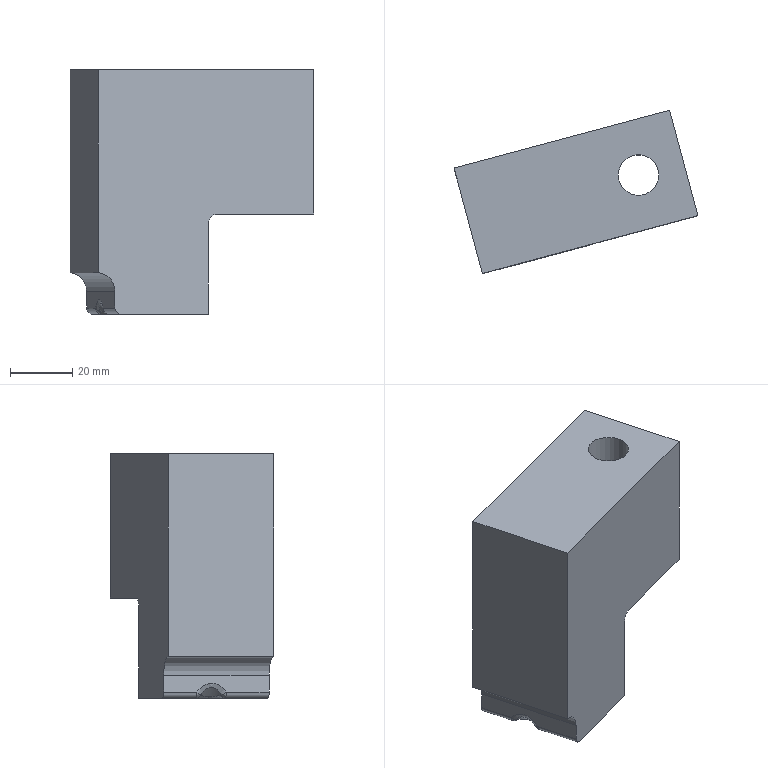Part | NX | features solid 2 | 1 solid | 27 faces | box 78.122 x 52.313 x 78.4 mm | volume 139499 mm3 | plane 12 | cylinder 10 | spline 4 | cone 1 | commonest cylinder face diameters 4 x2 6 x2 8.5 x1 10 x1 11 x1 12 x1
STEP:
#1=CARTESIAN_POINT('',(1284.025,27.373,18.75));
#2=VERTEX_POINT('',#1);
#3=CARTESIAN_POINT('',(1284.025,27.373,65.));
#4=VERTEX_POINT('',#3);
#5=CARTESIAN_POINT('',(1284.025,27.373,142.6));
#6=DIRECTION('',(0.,0.,-1.));
#7=VECTOR('',#6,1000.);
#8=LINE('',#5,#7);
#9=EDGE_CURVE('',#2,#4,#8,.F.);
#10=ORIENTED_EDGE('',*,*,#9,.T.);
#11=CARTESIAN_POINT('',(1214.961,8.867,65.));
#12=VERTEX_POINT('',#11);
#13=CARTESIAN_POINT('',(1303.344,32.549,65.));
#14=DIRECTION('',(-0.9659,-0.2588,0.));
#15=VECTOR('',#14,1000.);
#16=LINE('',#13,#15);
#17=EDGE_CURVE('',#4,#12,#16,.T.);
#18=ORIENTED_EDGE('',*,*,#17,.T.);
#19=CARTESIAN_POINT('',(1214.961,8.867,-0.02087));
#20=VERTEX_POINT('',#19);
#21=CARTESIAN_POINT('',(1214.961,8.867,86.));
#22=DIRECTION('',(0.,0.,1.));
#23=VECTOR('',#22,1000.);
#24=LINE('',#21,#23);
#25=EDGE_CURVE('',#20,#12,#24,.T.);
#26=ORIENTED_EDGE('',*,*,#25,.F.);
#27=CARTESIAN_POINT('',(1220.274,10.291,-6.));
#28=VERTEX_POINT('',#27);
#29=CARTESIAN_POINT('',(1214.478,8.738,-6.));
#30=DIRECTION('',(-0.2588,0.9659,0.));
#31=DIRECTION('',(-0.9659,-0.2588,0.));
#32=AXIS2_PLACEMENT_3D('',#29,#30,#31);
#33=CIRCLE('',#32,6.);
#34=EDGE_CURVE('',#20,#28,#33,.T.);
#35=ORIENTED_EDGE('',*,*,#34,.T.);
#36=CARTESIAN_POINT('',(1220.274,10.291,-11.4));
#37=VERTEX_POINT('',#36);
#38=CARTESIAN_POINT('',(1220.274,10.291,0.));
#39=DIRECTION('',(0.,0.,1.));
#40=VECTOR('',#39,1000.);
#41=LINE('',#38,#40);
#42=EDGE_CURVE('',#28,#37,#41,.F.);
#43=ORIENTED_EDGE('',*,*,#42,.T.);
#44=CARTESIAN_POINT('',(1222.206,10.808,-13.4));
#45=VERTEX_POINT('',#44);
#46=CARTESIAN_POINT('',(1222.206,10.808,-11.4));
#47=DIRECTION('',(-0.2588,0.9659,0.));
#48=DIRECTION('',(-0.9659,-0.2588,0.));
#49=AXIS2_PLACEMENT_3D('',#46,#47,#48);
#50=CIRCLE('',#49,2.);
#51=EDGE_CURVE('',#37,#45,#50,.F.);
#52=ORIENTED_EDGE('',*,*,#51,.T.);
#53=CARTESIAN_POINT('',(1250.218,18.314,-13.4));
#54=VERTEX_POINT('',#53);
#55=CARTESIAN_POINT('',(1303.344,32.549,-13.4));
#56=DIRECTION('',(0.9659,0.2588,0.));
#57=VECTOR('',#56,1000.);
#58=LINE('',#55,#57);
#59=EDGE_CURVE('',#54,#45,#58,.F.);
#60=ORIENTED_EDGE('',*,*,#59,.F.);
#61=CARTESIAN_POINT('',(1250.218,18.314,15.75));
#62=VERTEX_POINT('',#61);
#63=CARTESIAN_POINT('',(1250.218,18.314,142.6));
#64=DIRECTION('',(0.,0.,1.));
#65=VECTOR('',#64,1000.);
#66=LINE('',#63,#65);
#67=EDGE_CURVE('',#54,#62,#66,.T.);
#68=ORIENTED_EDGE('',*,*,#67,.T.);
#69=CARTESIAN_POINT('',(1253.115,19.091,18.75));
#70=VERTEX_POINT('',#69);
#71=CARTESIAN_POINT('',(1253.115,19.091,15.75));
#72=DIRECTION('',(0.2588,-0.9659,0.));
#73=DIRECTION('',(0.9659,0.2588,0.));
#74=AXIS2_PLACEMENT_3D('',#71,#72,#73);
#75=CIRCLE('',#74,3.);
#76=EDGE_CURVE('',#62,#70,#75,.F.);
#77=ORIENTED_EDGE('',*,*,#76,.T.);
#78=CARTESIAN_POINT('',(1303.344,32.549,18.75));
#79=DIRECTION('',(0.9659,0.2588,0.));
#80=VECTOR('',#79,1000.);
#81=LINE('',#78,#80);
#82=EDGE_CURVE('',#2,#70,#81,.F.);
#83=ORIENTED_EDGE('',*,*,#82,.F.);
#84=EDGE_LOOP('',(#10,#18,#26,#35,#43,#52,#60,#68,#77,#83));
#85=FACE_BOUND('',#84,.T.);
#86=CARTESIAN_POINT('',(1303.344,32.549,-6.));
#87=DIRECTION('',(0.2588,-0.9659,0.));
#88=DIRECTION('',(-0.9659,-0.2588,0.));
#89=AXIS2_PLACEMENT_3D('',#86,#87,#88);
#90=PLANE('',#89);
#91=ADVANCED_FACE('',(#85),#90,.T.);
#92=ORIENTED_EDGE('',*,*,#25,.T.);
#93=CARTESIAN_POINT('',(1205.903,42.675,65.));
#94=VERTEX_POINT('',#93);
#95=CARTESIAN_POINT('',(1203.025,53.415,65.));
#96=DIRECTION('',(-0.2588,0.9659,0.));
#97=VECTOR('',#96,1000.);
#98=LINE('',#95,#97);
#99=EDGE_CURVE('',#12,#94,#98,.T.);
#100=ORIENTED_EDGE('',*,*,#99,.T.);
#101=CARTESIAN_POINT('',(1205.903,42.675,-0.02087));
#102=VERTEX_POINT('',#101);
#103=CARTESIAN_POINT('',(1205.903,42.675,181.6));
#104=DIRECTION('',(0.,0.,-1.));
#105=VECTOR('',#104,1000.);
#106=LINE('',#103,#105);
#107=EDGE_CURVE('',#94,#102,#106,.T.);
#108=ORIENTED_EDGE('',*,*,#107,.T.);
#109=CARTESIAN_POINT('',(1215.168,8.097,-0.02087));
#110=DIRECTION('',(0.2588,-0.9659,0.));
#111=VECTOR('',#110,1000.);
#112=LINE('',#109,#111);
#113=EDGE_CURVE('',#20,#102,#112,.F.);
#114=ORIENTED_EDGE('',*,*,#113,.F.);
#115=EDGE_LOOP('',(#92,#100,#108,#114));
#116=FACE_BOUND('',#115,.T.);
#117=CARTESIAN_POINT('',(1203.025,53.415,86.));
#118=DIRECTION('',(-0.9659,-0.2588,0.));
#119=DIRECTION('',(-0.2588,0.9659,0.));
#120=AXIS2_PLACEMENT_3D('',#117,#118,#119);
#121=PLANE('',#120);
#122=ADVANCED_FACE('',(#116),#121,.T.);
#123=CARTESIAN_POINT('',(1274.966,61.18,65.));
#124=VERTEX_POINT('',#123);
#125=CARTESIAN_POINT('',(1213.147,44.616,65.));
#126=DIRECTION('',(-0.9659,-0.2588,0.));
#127=VECTOR('',#126,1000.);
#128=LINE('',#125,#127);
#129=EDGE_CURVE('',#124,#94,#128,.T.);
#130=ORIENTED_EDGE('',*,*,#129,.F.);
#131=CARTESIAN_POINT('',(1274.966,61.18,18.75));
#132=VERTEX_POINT('',#131);
#133=CARTESIAN_POINT('',(1274.966,61.18,142.6));
#134=DIRECTION('',(0.,0.,-1.));
#135=VECTOR('',#134,1000.);
#136=LINE('',#133,#135);
#137=EDGE_CURVE('',#132,#124,#136,.F.);
#138=ORIENTED_EDGE('',*,*,#137,.F.);
#139=CARTESIAN_POINT('',(1244.057,52.898,18.75));
#140=VERTEX_POINT('',#139);
#141=CARTESIAN_POINT('',(1213.147,44.616,18.75));
#142=DIRECTION('',(0.9659,0.2588,0.));
#143=VECTOR('',#142,1000.);
#144=LINE('',#141,#143);
#145=EDGE_CURVE('',#132,#140,#144,.F.);
#146=ORIENTED_EDGE('',*,*,#145,.T.);
#147=CARTESIAN_POINT('',(1241.159,52.122,15.75));
#148=VERTEX_POINT('',#147);
#149=CARTESIAN_POINT('',(1244.057,52.898,15.75));
#150=DIRECTION('',(0.2588,-0.9659,0.));
#151=DIRECTION('',(0.9659,0.2588,0.));
#152=AXIS2_PLACEMENT_3D('',#149,#150,#151);
#153=CIRCLE('',#152,3.);
#154=EDGE_CURVE('',#140,#148,#153,.T.);
#155=ORIENTED_EDGE('',*,*,#154,.T.);
#156=CARTESIAN_POINT('',(1241.159,52.122,-13.4));
#157=VERTEX_POINT('',#156);
#158=CARTESIAN_POINT('',(1241.159,52.122,142.6));
#159=DIRECTION('',(0.,0.,1.));
#160=VECTOR('',#159,1000.);
#161=LINE('',#158,#160);
#162=EDGE_CURVE('',#157,#148,#161,.T.);
#163=ORIENTED_EDGE('',*,*,#162,.F.);
#164=CARTESIAN_POINT('',(1213.147,44.616,-13.4));
#165=VERTEX_POINT('',#164);
#166=CARTESIAN_POINT('',(1211.215,44.098,-13.4));
#167=DIRECTION('',(-0.9659,-0.2588,0.));
#168=VECTOR('',#167,1000.);
#169=LINE('',#166,#168);
#170=EDGE_CURVE('',#157,#165,#169,.T.);
#171=ORIENTED_EDGE('',*,*,#170,.T.);
#172=CARTESIAN_POINT('',(1211.215,44.098,-11.4));
#173=VERTEX_POINT('',#172);
#174=CARTESIAN_POINT('',(1213.147,44.616,-11.4));
#175=DIRECTION('',(-0.2588,0.9659,0.));
#176=DIRECTION('',(-0.9659,-0.2588,0.));
#177=AXIS2_PLACEMENT_3D('',#174,#175,#176);
#178=CIRCLE('',#177,2.);
#179=EDGE_CURVE('',#173,#165,#178,.F.);
#180=ORIENTED_EDGE('',*,*,#179,.F.);
#181=CARTESIAN_POINT('',(1211.215,44.098,-6.));
#182=VERTEX_POINT('',#181);
#183=CARTESIAN_POINT('',(1211.215,44.098,0.));
#184=DIRECTION('',(0.,0.,1.));
#185=VECTOR('',#184,1000.);
#186=LINE('',#183,#185);
#187=EDGE_CURVE('',#173,#182,#186,.T.);
#188=ORIENTED_EDGE('',*,*,#187,.T.);
#189=CARTESIAN_POINT('',(1205.42,42.545,-6.));
#190=DIRECTION('',(-0.2588,0.9659,0.));
#191=DIRECTION('',(-0.9659,-0.2588,0.));
#192=AXIS2_PLACEMENT_3D('',#189,#190,#191);
#193=CIRCLE('',#192,6.);
#194=EDGE_CURVE('',#182,#102,#193,.F.);
#195=ORIENTED_EDGE('',*,*,#194,.T.);
#196=ORIENTED_EDGE('',*,*,#107,.F.);
#197=EDGE_LOOP('',(#130,#138,#146,#155,#163,#171,#180,#188,#195,#196));
#198=FACE_BOUND('',#197,.T.);
#199=CARTESIAN_POINT('',(1213.147,44.616,181.6));
#200=DIRECTION('',(0.2588,-0.9659,0.));
#201=DIRECTION('',(-0.9659,-0.2588,0.));
#202=AXIS2_PLACEMENT_3D('',#199,#200,#201);
#203=PLANE('',#202);
#204=ADVANCED_FACE('',(#198),#203,.F.);
#205=ORIENTED_EDGE('',*,*,#137,.T.);
#206=CARTESIAN_POINT('',(1284.231,26.602,65.));
#207=DIRECTION('',(0.2588,-0.9659,0.));
#208=VECTOR('',#207,1000.);
#209=LINE('',#206,#208);
#210=EDGE_CURVE('',#124,#4,#209,.T.);
#211=ORIENTED_EDGE('',*,*,#210,.T.);
#212=ORIENTED_EDGE('',*,*,#9,.F.);
#213=CARTESIAN_POINT('',(1284.231,26.602,18.75));
#214=DIRECTION('',(-0.2588,0.9659,0.));
#215=VECTOR('',#214,1000.);
#216=LINE('',#213,#215);
#217=EDGE_CURVE('',#132,#2,#216,.F.);
#218=ORIENTED_EDGE('',*,*,#217,.F.);
#219=EDGE_LOOP('',(#205,#211,#212,#218));
#220=FACE_BOUND('',#219,.T.);
#221=CARTESIAN_POINT('',(1284.231,26.602,142.6));
#222=DIRECTION('',(0.9659,0.2588,0.));
#223=DIRECTION('',(0.2588,-0.9659,0.));
#224=AXIS2_PLACEMENT_3D('',#221,#222,#223);
#225=PLANE('',#224);
#226=ADVANCED_FACE('',(#220),#225,.T.);
#227=CARTESIAN_POINT('',(1271.507,40.394,48.));
#228=VERTEX_POINT('',#227);
#229=CARTESIAN_POINT('',(1265.007,40.394,48.));
#230=DIRECTION('',(0.,0.,1.));
#231=DIRECTION('',(1.,0.,0.));
#232=AXIS2_PLACEMENT_3D('',#229,#230,#231);
#233=CIRCLE('',#232,6.5);
#234=EDGE_CURVE('',#228,#228,#233,.F.);
#235=ORIENTED_EDGE('',*,*,#234,.T.);
#236=EDGE_LOOP('',(#235));
#237=FACE_BOUND('',#236,.T.);
#238=CARTESIAN_POINT('',(1271.507,40.394,65.));
#239=VERTEX_POINT('',#238);
#240=CARTESIAN_POINT('',(1265.007,40.394,65.));
#241=DIRECTION('',(0.,0.,1.));
#242=DIRECTION('',(1.,0.,0.));
#243=AXIS2_PLACEMENT_3D('',#240,#241,#242);
#244=CIRCLE('',#243,6.5);
#245=EDGE_CURVE('',#239,#239,#244,.F.);
#246=ORIENTED_EDGE('',*,*,#245,.F.);
#247=EDGE_LOOP('',(#246));
#248=FACE_BOUND('',#247,.T.);
#249=CARTESIAN_POINT('',(1265.007,40.394,53.75));
#250=DIRECTION('',(0.,0.,1.));
#251=DIRECTION('',(1.,0.,0.));
#252=AXIS2_PLACEMENT_3D('',#249,#250,#251);
#253=CYLINDRICAL_SURFACE('',#252,6.5);
#254=ADVANCED_FACE('',(#237,#248),#253,.F.);
#255=CARTESIAN_POINT('',(1247.014,30.269,15.75));
#256=VERTEX_POINT('',#255);
#257=CARTESIAN_POINT('',(1247.014,30.269,-13.4));
#258=VERTEX_POINT('',#257);
#259=CARTESIAN_POINT('',(1247.014,30.269,18.75));
#260=DIRECTION('',(0.,0.,-1.));
#261=VECTOR('',#260,1000.);
#262=LINE('',#259,#261);
#263=EDGE_CURVE('',#256,#258,#262,.T.);
#264=ORIENTED_EDGE('',*,*,#263,.F.);
#265=CARTESIAN_POINT('',(1250.424,17.544,15.75));
#266=DIRECTION('',(-0.2588,0.9659,0.));
#267=VECTOR('',#266,1000.);
#268=LINE('',#265,#267);
#269=EDGE_CURVE('',#256,#62,#268,.F.);
#270=ORIENTED_EDGE('',*,*,#269,.T.);
#271=ORIENTED_EDGE('',*,*,#67,.F.);
#272=CARTESIAN_POINT('',(1242.3,47.861,-13.4));
#273=DIRECTION('',(0.2588,-0.9659,0.));
#274=VECTOR('',#273,1000.);
#275=LINE('',#272,#274);
#276=EDGE_CURVE('',#258,#54,#275,.T.);
#277=ORIENTED_EDGE('',*,*,#276,.F.);
#278=EDGE_LOOP('',(#264,#270,#271,#277));
#279=FACE_BOUND('',#278,.T.);
#280=CARTESIAN_POINT('',(1250.424,17.544,142.6));
#281=DIRECTION('',(0.9659,0.2588,0.));
#282=DIRECTION('',(0.2588,-0.9659,0.));
#283=AXIS2_PLACEMENT_3D('',#280,#281,#282);
#284=PLANE('',#283);
#285=ADVANCED_FACE('',(#279),#284,.T.);
#286=ORIENTED_EDGE('',*,*,#162,.T.);
#287=CARTESIAN_POINT('',(1244.362,40.167,15.75));
#288=VERTEX_POINT('',#287);
#289=CARTESIAN_POINT('',(1250.424,17.544,15.75));
#290=DIRECTION('',(-0.2588,0.9659,0.));
#291=VECTOR('',#290,1000.);
#292=LINE('',#289,#291);
#293=EDGE_CURVE('',#148,#288,#292,.F.);
#294=ORIENTED_EDGE('',*,*,#293,.T.);
#295=CARTESIAN_POINT('',(1244.362,40.167,-13.4));
#296=VERTEX_POINT('',#295);
#297=CARTESIAN_POINT('',(1244.362,40.167,-13.4));
#298=DIRECTION('',(0.,0.,-1.));
#299=VECTOR('',#298,1000.);
#300=LINE('',#297,#299);
#301=EDGE_CURVE('',#296,#288,#300,.F.);
#302=ORIENTED_EDGE('',*,*,#301,.F.);
#303=CARTESIAN_POINT('',(1242.3,47.861,-13.4));
#304=DIRECTION('',(0.2588,-0.9659,0.));
#305=VECTOR('',#304,1000.);
#306=LINE('',#303,#305);
#307=EDGE_CURVE('',#157,#296,#306,.T.);
#308=ORIENTED_EDGE('',*,*,#307,.F.);
#309=EDGE_LOOP('',(#286,#294,#302,#308));
#310=FACE_BOUND('',#309,.T.);
#311=CARTESIAN_POINT('',(1250.424,17.544,142.6));
#312=DIRECTION('',(0.9659,0.2588,0.));
#313=DIRECTION('',(0.2588,-0.9659,0.));
#314=AXIS2_PLACEMENT_3D('',#311,#312,#313);
#315=PLANE('',#314);
#316=ADVANCED_FACE('',(#310),#315,.T.);
#317=CARTESIAN_POINT('',(1217.195,25.606,-12.41));
#318=VERTEX_POINT('',#317);
#319=CARTESIAN_POINT('',(1216.601,23.998,-11.4));
#320=VERTEX_POINT('',#319);
#321=CARTESIAN_POINT('',(1217.195,25.606,-12.41));
#322=CARTESIAN_POINT('',(1217.092,25.518,-12.368));
#323=CARTESIAN_POINT('',(1216.836,25.249,-12.228));
#324=CARTESIAN_POINT('',(1216.559,24.723,-11.913));
#325=CARTESIAN_POINT('',(1216.534,24.249,-11.588));
#326=CARTESIAN_POINT('',(1216.601,23.998,-11.4));
#327=B_SPLINE_CURVE_WITH_KNOTS('',3,(#321,#322,#323,#324,#325,#326),.UNSPECIFIED.,.F.,.F.,(4,1,1,4),(0.,0.25,0.5,1.),.UNSPECIFIED.);
#328=EDGE_CURVE('',#318,#320,#327,.T.);
#329=ORIENTED_EDGE('',*,*,#328,.F.);
#330=CARTESIAN_POINT('',(1218.533,24.515,-13.4));
#331=VERTEX_POINT('',#330);
#332=CARTESIAN_POINT('',(1218.533,24.515,-13.4));
#333=CARTESIAN_POINT('',(1218.423,24.605,-13.4));
#334=CARTESIAN_POINT('',(1218.117,24.854,-13.353));
#335=CARTESIAN_POINT('',(1217.758,25.147,-13.159));
#336=CARTESIAN_POINT('',(1217.421,25.422,-12.819));
#337=CARTESIAN_POINT('',(1217.28,25.537,-12.597));
#338=CARTESIAN_POINT('',(1217.195,25.606,-12.41));
#339=B_SPLINE_CURVE_WITH_KNOTS('',3,(#332,#333,#334,#335,#336,#337,#338),.UNSPECIFIED.,.F.,.F.,(4,1,1,1,4),(0.,0.25,0.5,0.75,1.),.UNSPECIFIED.);
#340=EDGE_CURVE('',#318,#331,#339,.F.);
#341=ORIENTED_EDGE('',*,*,#340,.T.);
#342=CARTESIAN_POINT('',(1218.533,24.515,-11.4));
#343=DIRECTION('',(0.2588,-0.9659,0.));
#344=DIRECTION('',(-0.9659,-0.2588,0.));
#345=AXIS2_PLACEMENT_3D('',#342,#343,#344);
#346=CIRCLE('',#345,2.);
#347=EDGE_CURVE('',#331,#320,#346,.F.);
#348=ORIENTED_EDGE('',*,*,#347,.T.);
#349=EDGE_LOOP('',(#329,#341,#348));
#350=FACE_BOUND('',#349,.T.);
#351=CARTESIAN_POINT('',(1218.548,23.887,-13.299));
#352=CARTESIAN_POINT('',(1218.458,24.219,-13.409));
#353=CARTESIAN_POINT('',(1218.515,24.574,-13.431));
#354=CARTESIAN_POINT('',(1218.706,24.871,-13.36));
#355=CARTESIAN_POINT('',(1217.473,23.62,-13.219));
#356=CARTESIAN_POINT('',(1217.302,24.242,-13.426));
#357=CARTESIAN_POINT('',(1217.41,24.91,-13.468));
#358=CARTESIAN_POINT('',(1217.77,25.469,-13.335));
#359=CARTESIAN_POINT('',(1216.682,23.663,-12.44));
#360=CARTESIAN_POINT('',(1216.488,24.372,-12.676));
#361=CARTESIAN_POINT('',(1216.61,25.134,-12.723));
#362=CARTESIAN_POINT('',(1217.021,25.77,-12.571));
#363=CARTESIAN_POINT('',(1216.602,23.993,-11.382));
#364=CARTESIAN_POINT('',(1216.453,24.538,-11.563));
#365=CARTESIAN_POINT('',(1216.547,25.123,-11.6));
#366=CARTESIAN_POINT('',(1216.863,25.612,-11.483));
#367=(BOUNDED_SURFACE()B_SPLINE_SURFACE(3,3,((#351,#352,#353,#354),(#355,#356,#357,#358),(#359,#360,#361,#362),(#363,#364,#365,#366)),.UNSPECIFIED.,.F.,.F.,.F.)B_SPLINE_SURFACE_WITH_KNOTS((4,4),(4,4),(0.0005941,0.9994),(0.000239,0.9998),.PIECEWISE_BEZIER_KNOTS.)GEOMETRIC_REPRESENTATION_ITEM()RATIONAL_B_SPLINE_SURFACE(((0.9996,0.9224,0.9224,0.9996),(0.8197,0.7563,0.7563,0.8197),(0.8197,0.7563,0.7563,0.8197),(0.9996,0.9224,0.9224,0.9996)))REPRESENTATION_ITEM('')SURFACE());
#368=ADVANCED_FACE('',(#350),#367,.T.);
#369=CARTESIAN_POINT('',(1218.631,29.613,-12.814));
#370=VERTEX_POINT('',#369);
#371=CARTESIAN_POINT('',(1217.195,25.606,-12.41));
#372=CARTESIAN_POINT('',(1217.496,25.918,-12.472));
#373=CARTESIAN_POINT('',(1218.01,26.568,-12.582));
#374=CARTESIAN_POINT('',(1218.487,27.429,-12.697));
#375=CARTESIAN_POINT('',(1218.791,28.607,-12.796));
#376=CARTESIAN_POINT('',(1218.719,29.284,-12.814));
#377=CARTESIAN_POINT('',(1218.631,29.613,-12.814));
#378=B_SPLINE_CURVE_WITH_KNOTS('',3,(#371,#372,#373,#374,#375,#376,#377),.UNSPECIFIED.,.F.,.F.,(4,1,1,1,4),(0.000000039,0.25,0.5,0.75,1.),.UNSPECIFIED.);
#379=EDGE_CURVE('',#370,#318,#378,.F.);
#380=ORIENTED_EDGE('',*,*,#379,.T.);
#381=CARTESIAN_POINT('',(1215.899,28.881,-9.986));
#382=VERTEX_POINT('',#381);
#383=CARTESIAN_POINT('',(1215.899,28.881,-9.986));
#384=CARTESIAN_POINT('',(1215.99,28.54,-9.986));
#385=CARTESIAN_POINT('',(1216.196,27.854,-10.113));
#386=CARTESIAN_POINT('',(1216.544,26.924,-10.685));
#387=CARTESIAN_POINT('',(1216.844,26.251,-11.376));
#388=CARTESIAN_POINT('',(1217.077,25.806,-12.039));
#389=CARTESIAN_POINT('',(1217.195,25.606,-12.41));
#390=B_SPLINE_CURVE_WITH_KNOTS('',3,(#383,#384,#385,#386,#387,#388,#389),.UNSPECIFIED.,.F.,.F.,(4,1,1,1,4),(0.,0.25,0.5,0.75,1.),.UNSPECIFIED.);
#391=EDGE_CURVE('',#382,#318,#390,.T.);
#392=ORIENTED_EDGE('',*,*,#391,.F.);
#393=CARTESIAN_POINT('',(1215.384,32.366,-12.41));
#394=VERTEX_POINT('',#393);
#395=CARTESIAN_POINT('',(1215.899,28.881,-9.986));
#396=CARTESIAN_POINT('',(1215.716,29.563,-9.986));
#397=CARTESIAN_POINT('',(1215.439,30.969,-10.562));
#398=CARTESIAN_POINT('',(1215.38,31.927,-11.708));
#399=CARTESIAN_POINT('',(1215.384,32.366,-12.41));
#400=B_SPLINE_CURVE_WITH_KNOTS('',3,(#395,#396,#397,#398,#399),.UNSPECIFIED.,.F.,.F.,(4,1,4),(0.,0.5,1.),.UNSPECIFIED.);
#401=EDGE_CURVE('',#394,#382,#400,.F.);
#402=ORIENTED_EDGE('',*,*,#401,.F.);
#403=CARTESIAN_POINT('',(1218.631,29.613,-12.814));
#404=CARTESIAN_POINT('',(1218.543,29.942,-12.814));
#405=CARTESIAN_POINT('',(1218.266,30.564,-12.796));
#406=CARTESIAN_POINT('',(1217.414,31.433,-12.697));
#407=CARTESIAN_POINT('',(1216.571,31.94,-12.582));
#408=CARTESIAN_POINT('',(1215.801,32.246,-12.472));
#409=CARTESIAN_POINT('',(1215.384,32.366,-12.41));
#410=B_SPLINE_CURVE_WITH_KNOTS('',3,(#403,#404,#405,#406,#407,#408,#409),.UNSPECIFIED.,.F.,.F.,(4,1,1,1,4),(0.,0.25,0.5,0.75,1.),.UNSPECIFIED.);
#411=EDGE_CURVE('',#394,#370,#410,.F.);
#412=ORIENTED_EDGE('',*,*,#411,.T.);
#413=EDGE_LOOP('',(#380,#392,#402,#412));
#414=FACE_BOUND('',#413,.T.);
#415=CARTESIAN_POINT('',(1213.815,28.323,-14.899));
#416=DIRECTION('',(-0.683,-0.183,0.7071));
#417=DIRECTION('',(-0.683,-0.183,-0.7071));
#418=AXIS2_PLACEMENT_3D('',#415,#416,#417);
#419=CYLINDRICAL_SURFACE('',#418,5.);
#420=ADVANCED_FACE('',(#414),#419,.F.);
#421=CARTESIAN_POINT('',(1214.065,33.462,-11.4));
#422=VERTEX_POINT('',#421);
#423=CARTESIAN_POINT('',(1214.065,33.462,-11.4));
#424=CARTESIAN_POINT('',(1214.095,33.351,-11.483));
#425=CARTESIAN_POINT('',(1214.223,33.054,-11.714));
#426=CARTESIAN_POINT('',(1214.507,32.741,-11.985));
#427=CARTESIAN_POINT('',(1214.927,32.488,-12.24));
#428=CARTESIAN_POINT('',(1215.18,32.403,-12.346));
#429=CARTESIAN_POINT('',(1215.384,32.366,-12.41));
#430=B_SPLINE_CURVE_WITH_KNOTS('',3,(#423,#424,#425,#426,#427,#428,#429),.UNSPECIFIED.,.F.,.F.,(4,1,1,1,4),(0.,0.25,0.5,0.75,1.),.UNSPECIFIED.);
#431=EDGE_CURVE('',#422,#394,#430,.T.);
#432=ORIENTED_EDGE('',*,*,#431,.F.);
#433=CARTESIAN_POINT('',(1215.997,33.979,-13.4));
#434=VERTEX_POINT('',#433);
#435=CARTESIAN_POINT('',(1215.997,33.979,-11.4));
#436=DIRECTION('',(-0.2588,0.9659,0.));
#437=DIRECTION('',(-0.9659,-0.2588,0.));
#438=AXIS2_PLACEMENT_3D('',#435,#436,#437);
#439=CIRCLE('',#438,2.);
#440=EDGE_CURVE('',#422,#434,#439,.F.);
#441=ORIENTED_EDGE('',*,*,#440,.T.);
#442=CARTESIAN_POINT('',(1215.384,32.366,-12.41));
#443=CARTESIAN_POINT('',(1215.409,32.432,-12.532));
#444=CARTESIAN_POINT('',(1215.494,32.656,-12.849));
#445=CARTESIAN_POINT('',(1215.685,33.159,-13.253));
#446=CARTESIAN_POINT('',(1215.883,33.679,-13.4));
#447=CARTESIAN_POINT('',(1215.997,33.979,-13.4));
#448=B_SPLINE_CURVE_WITH_KNOTS('',3,(#442,#443,#444,#445,#446,#447),.UNSPECIFIED.,.F.,.F.,(4,1,1,4),(0.,0.25,0.5,1.),.UNSPECIFIED.);
#449=EDGE_CURVE('',#434,#394,#448,.F.);
#450=ORIENTED_EDGE('',*,*,#449,.T.);
#451=EDGE_LOOP('',(#432,#441,#450));
#452=FACE_BOUND('',#451,.T.);
#453=CARTESIAN_POINT('',(1214.005,34.078,-11.546));
#454=CARTESIAN_POINT('',(1213.987,33.718,-11.548));
#455=CARTESIAN_POINT('',(1214.051,33.395,-11.401));
#456=CARTESIAN_POINT('',(1214.181,33.184,-11.139));
#457=CARTESIAN_POINT('',(1214.086,34.079,-12.656));
#458=CARTESIAN_POINT('',(1214.053,33.402,-12.659));
#459=CARTESIAN_POINT('',(1214.173,32.794,-12.383));
#460=CARTESIAN_POINT('',(1214.417,32.397,-11.89));
#461=CARTESIAN_POINT('',(1214.904,34.043,-13.41));
#462=CARTESIAN_POINT('',(1214.866,33.271,-13.414));
#463=CARTESIAN_POINT('',(1215.002,32.578,-13.098));
#464=CARTESIAN_POINT('',(1215.281,32.126,-12.536));
#465=CARTESIAN_POINT('',(1216.015,33.989,-13.4));
#466=CARTESIAN_POINT('',(1215.986,33.396,-13.403));
#467=CARTESIAN_POINT('',(1216.091,32.864,-13.161));
#468=CARTESIAN_POINT('',(1216.305,32.517,-12.729));
#469=(BOUNDED_SURFACE()B_SPLINE_SURFACE(3,3,((#453,#454,#455,#456),(#457,#458,#459,#460),(#461,#462,#463,#464),(#465,#466,#467,#468)),.UNSPECIFIED.,.F.,.F.,.F.)B_SPLINE_SURFACE_WITH_KNOTS((4,4),(4,4),(0.,1.),(0.,1.),.PIECEWISE_BEZIER_KNOTS.)GEOMETRIC_REPRESENTATION_ITEM()RATIONAL_B_SPLINE_SURFACE(((1.,0.9226,0.9226,1.),(0.8196,0.7562,0.7562,0.8196),(0.8196,0.7562,0.7562,0.8196),(1.,0.9226,0.9226,1.)))REPRESENTATION_ITEM('')SURFACE());
#470=ADVANCED_FACE('',(#452),#469,.T.);
#471=ORIENTED_EDGE('',*,*,#431,.T.);
#472=ORIENTED_EDGE('',*,*,#401,.T.);
#473=ORIENTED_EDGE('',*,*,#391,.T.);
#474=ORIENTED_EDGE('',*,*,#328,.T.);
#475=CARTESIAN_POINT('',(1214.065,33.462,-11.4));
#476=CARTESIAN_POINT('',(1214.141,33.181,-10.997));
#477=CARTESIAN_POINT('',(1214.303,32.574,-10.273));
#478=CARTESIAN_POINT('',(1214.581,31.538,-9.387));
#479=CARTESIAN_POINT('',(1214.975,30.067,-8.69));
#480=CARTESIAN_POINT('',(1215.325,28.758,-8.504));
#481=CARTESIAN_POINT('',(1215.724,27.272,-8.723));
#482=CARTESIAN_POINT('',(1216.189,25.536,-9.585));
#483=CARTESIAN_POINT('',(1216.451,24.557,-10.597));
#484=CARTESIAN_POINT('',(1216.601,23.998,-11.4));
#485=B_SPLINE_CURVE_WITH_KNOTS('',3,(#475,#476,#477,#478,#479,#480,#481,#482,#483,#484),.UNSPECIFIED.,.F.,.F.,(4,1,1,1,1,1,1,4),(0.,0.125,0.25,0.375,0.5,0.625,0.75,1.),.UNSPECIFIED.);
#486=EDGE_CURVE('',#320,#422,#485,.F.);
#487=ORIENTED_EDGE('',*,*,#486,.T.);
#488=EDGE_LOOP('',(#471,#472,#473,#474,#487));
#489=FACE_BOUND('',#488,.T.);
#490=CARTESIAN_POINT('',(1216.613,23.952,-11.464));
#491=CARTESIAN_POINT('',(1216.369,24.862,-12.132));
#492=CARTESIAN_POINT('',(1217.213,25.576,-12.466));
#493=CARTESIAN_POINT('',(1216.278,25.204,-9.636));
#494=CARTESIAN_POINT('',(1216.13,25.757,-10.49));
#495=CARTESIAN_POINT('',(1216.721,26.403,-10.898));
#496=CARTESIAN_POINT('',(1215.333,28.73,-7.507));
#497=CARTESIAN_POINT('',(1215.333,28.73,-8.356));
#498=CARTESIAN_POINT('',(1215.752,28.842,-9.074));
#499=CARTESIAN_POINT('',(1214.388,32.255,-9.636));
#500=CARTESIAN_POINT('',(1214.537,31.702,-10.49));
#501=CARTESIAN_POINT('',(1215.372,31.439,-10.898));
#502=CARTESIAN_POINT('',(1214.053,33.507,-11.464));
#503=CARTESIAN_POINT('',(1214.297,32.597,-12.132));
#504=CARTESIAN_POINT('',(1215.384,32.4,-12.466));
#505=(BOUNDED_SURFACE()B_SPLINE_SURFACE(3,2,((#490,#491,#492),(#493,#494,#495),(#496,#497,#498),(#499,#500,#501),(#502,#503,#504)),.UNSPECIFIED.,.F.,.F.,.F.)B_SPLINE_SURFACE_WITH_KNOTS((4,1,4),(3,3),(5.499,6.283,7.068),(0.,1.),.UNSPECIFIED.)GEOMETRIC_REPRESENTATION_ITEM()RATIONAL_B_SPLINE_SURFACE(((1.,0.8662,1.),(1.,0.9039,1.),(1.,0.9439,1.),(1.,0.9039,1.),(1.,0.8662,1.)))REPRESENTATION_ITEM('')SURFACE());
#506=ADVANCED_FACE('',(#489),#505,.T.);
#507=CARTESIAN_POINT('',(1215.255,36.748,-13.4));
#508=DIRECTION('',(0.2588,-0.9659,0.));
#509=VECTOR('',#508,1000.);
#510=LINE('',#507,#509);
#511=EDGE_CURVE('',#331,#45,#510,.T.);
#512=ORIENTED_EDGE('',*,*,#511,.T.);
#513=ORIENTED_EDGE('',*,*,#51,.F.);
#514=CARTESIAN_POINT('',(1208.337,54.839,-11.4));
#515=DIRECTION('',(-0.2588,0.9659,0.));
#516=VECTOR('',#515,1000.);
#517=LINE('',#514,#516);
#518=EDGE_CURVE('',#37,#320,#517,.T.);
#519=ORIENTED_EDGE('',*,*,#518,.T.);
#520=ORIENTED_EDGE('',*,*,#347,.F.);
#521=EDGE_LOOP('',(#512,#513,#519,#520));
#522=FACE_BOUND('',#521,.T.);
#523=CARTESIAN_POINT('',(1215.255,36.748,-11.4));
#524=DIRECTION('',(0.2588,-0.9659,0.));
#525=DIRECTION('',(0.9659,0.2588,0.));
#526=AXIS2_PLACEMENT_3D('',#523,#524,#525);
#527=CYLINDRICAL_SURFACE('',#526,2.);
#528=ADVANCED_FACE('',(#522),#527,.T.);
#529=ORIENTED_EDGE('',*,*,#379,.F.);
#530=ORIENTED_EDGE('',*,*,#411,.F.);
#531=ORIENTED_EDGE('',*,*,#449,.F.);
#532=CARTESIAN_POINT('',(1218.533,24.515,-13.4));
#533=CARTESIAN_POINT('',(1218.674,24.688,-13.4));
#534=CARTESIAN_POINT('',(1218.87,24.947,-13.4));
#535=CARTESIAN_POINT('',(1219.116,25.318,-13.4));
#536=CARTESIAN_POINT('',(1219.262,25.552,-13.4));
#537=CARTESIAN_POINT('',(1219.491,25.972,-13.4));
#538=CARTESIAN_POINT('',(1219.642,26.288,-13.4));
#539=CARTESIAN_POINT('',(1219.872,26.858,-13.4));
#540=CARTESIAN_POINT('',(1220.033,27.454,-13.4));
#541=CARTESIAN_POINT('',(1220.082,27.715,-13.4));
#542=CARTESIAN_POINT('',(1220.153,28.177,-13.4));
#543=CARTESIAN_POINT('',(1220.191,28.931,-13.4));
#544=CARTESIAN_POINT('',(1220.078,29.785,-13.4));
#545=CARTESIAN_POINT('',(1219.84,30.483,-13.4));
#546=CARTESIAN_POINT('',(1219.676,30.855,-13.4));
#547=CARTESIAN_POINT('',(1219.506,31.175,-13.4));
#548=CARTESIAN_POINT('',(1219.427,31.305,-13.4));
#549=CARTESIAN_POINT('',(1219.318,31.478,-13.4));
#550=CARTESIAN_POINT('',(1219.195,31.652,-13.4));
#551=CARTESIAN_POINT('',(1219.117,31.763,-13.4));
#552=CARTESIAN_POINT('',(1218.836,32.106,-13.4));
#553=CARTESIAN_POINT('',(1218.584,32.369,-13.4));
#554=CARTESIAN_POINT('',(1218.287,32.644,-13.4));
#555=CARTESIAN_POINT('',(1218.013,32.871,-13.4));
#556=CARTESIAN_POINT('',(1217.557,33.199,-13.4));
#557=CARTESIAN_POINT('',(1216.981,33.549,-13.4));
#558=CARTESIAN_POINT('',(1216.389,33.83,-13.4));
#559=CARTESIAN_POINT('',(1215.997,33.979,-13.4));
#560=B_SPLINE_CURVE_WITH_KNOTS('',3,(#532,#533,#534,#535,#536,#537,#538,#539,#540,#541,#542,#543,#544,#545,#546,#547,#548,#549,#550,#551,#552,#553,#554,#555,#556,#557,#558,#559),.UNSPECIFIED.,.F.,.F.,(4,1,1,1,1,1,1,1,1,1,1,1,1,1,1,1,1,1,1,1,1,1,1,1,1,4),(0.,0.0625,0.09375,0.125,0.1562,0.1875,0.2188,0.25,0.2812,0.3125,0.375,0.5,0.5625,0.5938,0.625,0.6562,0.6875,0.7188,0.75,0.7812,0.8125,0.8438,0.875,0.9062,0.9375,1.),.UNSPECIFIED.);
#561=EDGE_CURVE('',#434,#331,#560,.F.);
#562=ORIENTED_EDGE('',*,*,#561,.T.);
#563=ORIENTED_EDGE('',*,*,#340,.F.);
#564=EDGE_LOOP('',(#529,#530,#531,#562,#563));
#565=FACE_BOUND('',#564,.T.);
#566=CARTESIAN_POINT('',(1215.923,34.008,-13.4));
#567=CARTESIAN_POINT('',(1215.522,32.925,-13.4));
#568=CARTESIAN_POINT('',(1215.321,32.383,-12.4));
#569=CARTESIAN_POINT('',(1218.025,33.23,-13.4));
#570=CARTESIAN_POINT('',(1217.347,32.455,-13.4));
#571=CARTESIAN_POINT('',(1217.075,31.895,-12.662));
#572=CARTESIAN_POINT('',(1221.026,30.255,-13.4));
#573=CARTESIAN_POINT('',(1220.206,30.035,-13.4));
#574=CARTESIAN_POINT('',(1219.512,29.849,-12.966));
#575=CARTESIAN_POINT('',(1219.914,26.178,-13.4));
#576=CARTESIAN_POINT('',(1218.94,26.51,-13.4));
#577=CARTESIAN_POINT('',(1218.424,26.859,-12.662));
#578=CARTESIAN_POINT('',(1218.483,24.453,-13.4));
#579=CARTESIAN_POINT('',(1217.594,25.191,-13.4));
#580=CARTESIAN_POINT('',(1217.15,25.56,-12.4));
#581=(BOUNDED_SURFACE()B_SPLINE_SURFACE(3,2,((#566,#567,#568),(#569,#570,#571),(#572,#573,#574),(#575,#576,#577),(#578,#579,#580)),.UNSPECIFIED.,.F.,.F.,.F.)B_SPLINE_SURFACE_WITH_KNOTS((4,1,4),(3,3),(2.357,3.142,3.926),(0.,1.),.UNSPECIFIED.)GEOMETRIC_REPRESENTATION_ITEM()RATIONAL_B_SPLINE_SURFACE(((1.,0.8662,1.),(1.,0.9039,1.),(1.,0.9439,1.),(1.,0.9039,1.),(1.,0.8662,1.)))REPRESENTATION_ITEM('')SURFACE());
#582=ADVANCED_FACE('',(#565),#581,.T.);
#583=CARTESIAN_POINT('',(1204.828,67.934,-6.));
#584=DIRECTION('',(0.2588,-0.9659,0.));
#585=VECTOR('',#584,1000.);
#586=LINE('',#583,#585);
#587=EDGE_CURVE('',#28,#182,#586,.F.);
#588=ORIENTED_EDGE('',*,*,#587,.F.);
#589=ORIENTED_EDGE('',*,*,#34,.F.);
#590=ORIENTED_EDGE('',*,*,#113,.T.);
#591=ORIENTED_EDGE('',*,*,#194,.F.);
#592=EDGE_LOOP('',(#588,#589,#590,#591));
#593=FACE_BOUND('',#592,.T.);
#594=CARTESIAN_POINT('',(1199.033,66.381,-6.));
#595=DIRECTION('',(0.2588,-0.9659,0.));
#596=DIRECTION('',(0.9659,0.2588,0.));
#597=AXIS2_PLACEMENT_3D('',#594,#595,#596);
#598=CYLINDRICAL_SURFACE('',#597,6.);
#599=ADVANCED_FACE('',(#593),#598,.F.);
#600=ORIENTED_EDGE('',*,*,#307,.T.);
#601=CARTESIAN_POINT('',(1247.62,35.735,-13.4));
#602=DIRECTION('',(0.,0.,1.));
#603=DIRECTION('',(1.,0.,0.));
#604=AXIS2_PLACEMENT_3D('',#601,#602,#603);
#605=CIRCLE('',#604,5.5);
#606=EDGE_CURVE('',#296,#258,#605,.T.);
#607=ORIENTED_EDGE('',*,*,#606,.T.);
#608=ORIENTED_EDGE('',*,*,#276,.T.);
#609=ORIENTED_EDGE('',*,*,#59,.T.);
#610=ORIENTED_EDGE('',*,*,#511,.F.);
#611=ORIENTED_EDGE('',*,*,#561,.F.);
#612=CARTESIAN_POINT('',(1215.255,36.748,-13.4));
#613=DIRECTION('',(0.2588,-0.9659,0.));
#614=VECTOR('',#613,1000.);
#615=LINE('',#612,#614);
#616=EDGE_CURVE('',#165,#434,#615,.T.);
#617=ORIENTED_EDGE('',*,*,#616,.F.);
#618=ORIENTED_EDGE('',*,*,#170,.F.);
#619=EDGE_LOOP('',(#600,#607,#608,#609,#610,#611,#617,#618));
#620=FACE_BOUND('',#619,.T.);
#621=CARTESIAN_POINT('',(1212.357,39.838,-13.4));
#622=DIRECTION('',(0.,0.,1.));
#623=DIRECTION('',(-0.2588,0.9659,0.));
#624=AXIS2_PLACEMENT_3D('',#621,#622,#623);
#625=PLANE('',#624);
#626=ADVANCED_FACE('',(#620),#625,.F.);
#627=CARTESIAN_POINT('',(1208.337,54.839,-11.4));
#628=DIRECTION('',(-0.2588,0.9659,0.));
#629=VECTOR('',#628,1000.);
#630=LINE('',#627,#629);
#631=EDGE_CURVE('',#422,#173,#630,.T.);
#632=ORIENTED_EDGE('',*,*,#631,.F.);
#633=ORIENTED_EDGE('',*,*,#486,.F.);
#634=ORIENTED_EDGE('',*,*,#518,.F.);
#635=ORIENTED_EDGE('',*,*,#42,.F.);
#636=ORIENTED_EDGE('',*,*,#587,.T.);
#637=ORIENTED_EDGE('',*,*,#187,.F.);
#638=EDGE_LOOP('',(#632,#633,#634,#635,#636,#637));
#639=FACE_BOUND('',#638,.T.);
#640=CARTESIAN_POINT('',(1208.337,54.839,0.));
#641=DIRECTION('',(0.9659,0.2588,0.));
#642=DIRECTION('',(0.,0.,1.));
#643=AXIS2_PLACEMENT_3D('',#640,#641,#642);
#644=PLANE('',#643);
#645=ADVANCED_FACE('',(#639),#644,.F.);
#646=ORIENTED_EDGE('',*,*,#179,.T.);
#647=ORIENTED_EDGE('',*,*,#616,.T.);
#648=ORIENTED_EDGE('',*,*,#440,.F.);
#649=ORIENTED_EDGE('',*,*,#631,.T.);
#650=EDGE_LOOP('',(#646,#647,#648,#649));
#651=FACE_BOUND('',#650,.T.);
#652=CARTESIAN_POINT('',(1215.255,36.748,-11.4));
#653=DIRECTION('',(0.2588,-0.9659,0.));
#654=DIRECTION('',(0.9659,0.2588,0.));
#655=AXIS2_PLACEMENT_3D('',#652,#653,#654);
#656=CYLINDRICAL_SURFACE('',#655,2.);
#657=ADVANCED_FACE('',(#651),#656,.T.);
#658=CARTESIAN_POINT('',(1275.007,40.394,18.75));
#659=VERTEX_POINT('',#658);
#660=CARTESIAN_POINT('',(1265.007,40.394,18.75));
#661=DIRECTION('',(0.,0.,1.));
#662=DIRECTION('',(1.,0.,0.));
#663=AXIS2_PLACEMENT_3D('',#660,#661,#662);
#664=CIRCLE('',#663,10.);
#665=EDGE_CURVE('',#659,#659,#664,.T.);
#666=ORIENTED_EDGE('',*,*,#665,.T.);
#667=EDGE_LOOP('',(#666));
#668=FACE_BOUND('',#667,.T.);
#669=CARTESIAN_POINT('',(1249.986,30.77,18.75));
#670=VERTEX_POINT('',#669);
#671=CARTESIAN_POINT('',(1247.186,41.218,18.75));
#672=VERTEX_POINT('',#671);
#673=CARTESIAN_POINT('',(1247.62,35.735,18.75));
#674=DIRECTION('',(0.,0.,-1.));
#675=DIRECTION('',(-1.,0.,0.));
#676=AXIS2_PLACEMENT_3D('',#673,#674,#675);
#677=CIRCLE('',#676,5.5);
#678=EDGE_CURVE('',#670,#672,#677,.F.);
#679=ORIENTED_EDGE('',*,*,#678,.T.);
#680=CARTESIAN_POINT('',(1213.723,166.104,18.75));
#681=DIRECTION('',(0.2588,-0.9659,0.));
#682=VECTOR('',#681,1000.);
#683=LINE('',#680,#682);
#684=EDGE_CURVE('',#672,#140,#683,.F.);
#685=ORIENTED_EDGE('',*,*,#684,.T.);
#686=ORIENTED_EDGE('',*,*,#145,.F.);
#687=ORIENTED_EDGE('',*,*,#217,.T.);
#688=ORIENTED_EDGE('',*,*,#82,.T.);
#689=CARTESIAN_POINT('',(1213.723,166.104,18.75));
#690=DIRECTION('',(0.2588,-0.9659,0.));
#691=VECTOR('',#690,1000.);
#692=LINE('',#689,#691);
#693=EDGE_CURVE('',#70,#670,#692,.F.);
#694=ORIENTED_EDGE('',*,*,#693,.T.);
#695=EDGE_LOOP('',(#679,#685,#686,#687,#688,#694));
#696=FACE_BOUND('',#695,.T.);
#697=CARTESIAN_POINT('',(1187.786,159.154,18.75));
#698=DIRECTION('',(0.,0.,-1.));
#699=DIRECTION('',(-1.,0.,0.));
#700=AXIS2_PLACEMENT_3D('',#697,#698,#699);
#701=PLANE('',#700);
#702=ADVANCED_FACE('',(#668,#696),#701,.T.);
#703=ORIENTED_EDGE('',*,*,#234,.F.);
#704=EDGE_LOOP('',(#703));
#705=FACE_BOUND('',#704,.T.);
#706=CARTESIAN_POINT('',(1275.007,40.394,48.));
#707=VERTEX_POINT('',#706);
#708=CARTESIAN_POINT('',(1265.007,40.394,48.));
#709=DIRECTION('',(0.,0.,1.));
#710=DIRECTION('',(1.,0.,0.));
#711=AXIS2_PLACEMENT_3D('',#708,#709,#710);
#712=CIRCLE('',#711,10.);
#713=EDGE_CURVE('',#707,#707,#712,.F.);
#714=ORIENTED_EDGE('',*,*,#713,.T.);
#715=EDGE_LOOP('',(#714));
#716=FACE_BOUND('',#715,.T.);
#717=CARTESIAN_POINT('',(1265.007,40.394,48.));
#718=DIRECTION('',(0.,0.,1.));
#719=DIRECTION('',(1.,0.,0.));
#720=AXIS2_PLACEMENT_3D('',#717,#718,#719);
#721=PLANE('',#720);
#722=ADVANCED_FACE('',(#705,#716),#721,.F.);
#723=ORIENTED_EDGE('',*,*,#713,.F.);
#724=EDGE_LOOP('',(#723));
#725=FACE_BOUND('',#724,.T.);
#726=ORIENTED_EDGE('',*,*,#665,.F.);
#727=EDGE_LOOP('',(#726));
#728=FACE_BOUND('',#727,.T.);
#729=CARTESIAN_POINT('',(1265.007,40.394,18.75));
#730=DIRECTION('',(0.,0.,1.));
#731=DIRECTION('',(1.,0.,0.));
#732=AXIS2_PLACEMENT_3D('',#729,#730,#731);
#733=CYLINDRICAL_SURFACE('',#732,10.);
#734=ADVANCED_FACE('',(#725,#728),#733,.F.);
#735=CARTESIAN_POINT('',(1242.12,35.735,28.75));
#736=VERTEX_POINT('',#735);
#737=CARTESIAN_POINT('',(1247.62,35.735,28.75));
#738=DIRECTION('',(0.,0.,-1.));
#739=DIRECTION('',(-1.,0.,0.));
#740=AXIS2_PLACEMENT_3D('',#737,#738,#739);
#741=CIRCLE('',#740,5.5);
#742=EDGE_CURVE('',#736,#736,#741,.F.);
#743=ORIENTED_EDGE('',*,*,#742,.T.);
#744=EDGE_LOOP('',(#743));
#745=FACE_BOUND('',#744,.T.);
#746=ORIENTED_EDGE('',*,*,#301,.T.);
#747=CARTESIAN_POINT('',(1244.362,40.167,15.75));
#748=CARTESIAN_POINT('',(1244.362,40.167,16.548));
#749=CARTESIAN_POINT('',(1244.907,40.63,18.09));
#750=CARTESIAN_POINT('',(1246.39,41.155,18.75));
#751=CARTESIAN_POINT('',(1247.186,41.218,18.75));
#752=B_SPLINE_CURVE_WITH_KNOTS('',3,(#747,#748,#749,#750,#751),.UNSPECIFIED.,.F.,.F.,(4,1,4),(0.,0.002358,0.004715),.UNSPECIFIED.);
#753=EDGE_CURVE('',#288,#672,#752,.T.);
#754=ORIENTED_EDGE('',*,*,#753,.T.);
#755=ORIENTED_EDGE('',*,*,#678,.F.);
#756=CARTESIAN_POINT('',(1249.986,30.77,18.75));
#757=CARTESIAN_POINT('',(1249.265,30.427,18.75));
#758=CARTESIAN_POINT('',(1247.717,30.14,18.089));
#759=CARTESIAN_POINT('',(1247.014,30.269,16.548));
#760=CARTESIAN_POINT('',(1247.014,30.269,15.75));
#761=B_SPLINE_CURVE_WITH_KNOTS('',3,(#756,#757,#758,#759,#760),.UNSPECIFIED.,.F.,.F.,(4,1,4),(0.,0.002359,0.004718),.UNSPECIFIED.);
#762=EDGE_CURVE('',#670,#256,#761,.T.);
#763=ORIENTED_EDGE('',*,*,#762,.T.);
#764=ORIENTED_EDGE('',*,*,#263,.T.);
#765=ORIENTED_EDGE('',*,*,#606,.F.);
#766=EDGE_LOOP('',(#746,#754,#755,#763,#764,#765));
#767=FACE_BOUND('',#766,.T.);
#768=CARTESIAN_POINT('',(1247.62,35.735,33.75));
#769=DIRECTION('',(0.,0.,-1.));
#770=DIRECTION('',(-1.,0.,0.));
#771=AXIS2_PLACEMENT_3D('',#768,#769,#770);
#772=CYLINDRICAL_SURFACE('',#771,5.5);
#773=ADVANCED_FACE('',(#745,#767),#772,.F.);
#774=CARTESIAN_POINT('',(1251.87,35.735,28.75));
#775=VERTEX_POINT('',#774);
#776=CARTESIAN_POINT('',(1247.62,35.735,28.75));
#777=DIRECTION('',(0.,0.,1.));
#778=DIRECTION('',(1.,0.,0.));
#779=AXIS2_PLACEMENT_3D('',#776,#777,#778);
#780=CIRCLE('',#779,4.25);
#781=EDGE_CURVE('',#775,#775,#780,.T.);
#782=ORIENTED_EDGE('',*,*,#781,.T.);
#783=EDGE_LOOP('',(#782));
#784=FACE_BOUND('',#783,.T.);
#785=ORIENTED_EDGE('',*,*,#742,.F.);
#786=EDGE_LOOP('',(#785));
#787=FACE_BOUND('',#786,.T.);
#788=CARTESIAN_POINT('',(1247.62,35.735,28.75));
#789=DIRECTION('',(0.,0.,-1.));
#790=DIRECTION('',(-1.,0.,0.));
#791=AXIS2_PLACEMENT_3D('',#788,#789,#790);
#792=PLANE('',#791);
#793=ADVANCED_FACE('',(#784,#787),#792,.T.);
#794=CARTESIAN_POINT('',(1251.87,35.735,58.75));
#795=VERTEX_POINT('',#794);
#796=CARTESIAN_POINT('',(1247.62,35.735,58.75));
#797=DIRECTION('',(0.,0.,1.));
#798=DIRECTION('',(1.,0.,0.));
#799=AXIS2_PLACEMENT_3D('',#796,#797,#798);
#800=CIRCLE('',#799,4.25);
#801=EDGE_CURVE('',#795,#795,#800,.F.);
#802=ORIENTED_EDGE('',*,*,#801,.T.);
#803=EDGE_LOOP('',(#802));
#804=FACE_BOUND('',#803,.T.);
#805=CARTESIAN_POINT('',(1247.62,35.735,61.304));
#806=VERTEX_POINT('',#805);
#807=VERTEX_LOOP('',#806);
#808=FACE_BOUND('',#807,.T.);
#809=CARTESIAN_POINT('',(1247.62,35.735,58.75));
#810=DIRECTION('',(0.,0.,-1.));
#811=DIRECTION('',(-1.,0.,0.));
#812=AXIS2_PLACEMENT_3D('',#809,#810,#811);
#813=CONICAL_SURFACE('',#812,4.25,1.03);
#814=ADVANCED_FACE('',(#804,#808),#813,.F.);
#815=ORIENTED_EDGE('',*,*,#801,.F.);
#816=EDGE_LOOP('',(#815));
#817=FACE_BOUND('',#816,.T.);
#818=ORIENTED_EDGE('',*,*,#781,.F.);
#819=EDGE_LOOP('',(#818));
#820=FACE_BOUND('',#819,.T.);
#821=CARTESIAN_POINT('',(1247.62,35.735,33.75));
#822=DIRECTION('',(0.,0.,1.));
#823=DIRECTION('',(1.,0.,0.));
#824=AXIS2_PLACEMENT_3D('',#821,#822,#823);
#825=CYLINDRICAL_SURFACE('',#824,4.25);
#826=ADVANCED_FACE('',(#817,#820),#825,.F.);
#827=ORIENTED_EDGE('',*,*,#154,.F.);
#828=ORIENTED_EDGE('',*,*,#684,.F.);
#829=ORIENTED_EDGE('',*,*,#753,.F.);
#830=ORIENTED_EDGE('',*,*,#293,.F.);
#831=EDGE_LOOP('',(#827,#828,#829,#830));
#832=FACE_BOUND('',#831,.T.);
#833=CARTESIAN_POINT('',(1253.322,18.32,15.75));
#834=DIRECTION('',(-0.2588,0.9659,0.));
#835=DIRECTION('',(-0.9659,-0.2588,0.));
#836=AXIS2_PLACEMENT_3D('',#833,#834,#835);
#837=CYLINDRICAL_SURFACE('',#836,3.);
#838=ADVANCED_FACE('',(#832),#837,.F.);
#839=ORIENTED_EDGE('',*,*,#762,.F.);
#840=ORIENTED_EDGE('',*,*,#693,.F.);
#841=ORIENTED_EDGE('',*,*,#76,.F.);
#842=ORIENTED_EDGE('',*,*,#269,.F.);
#843=EDGE_LOOP('',(#839,#840,#841,#842));
#844=FACE_BOUND('',#843,.T.);
#845=CARTESIAN_POINT('',(1253.322,18.32,15.75));
#846=DIRECTION('',(-0.2588,0.9659,0.));
#847=DIRECTION('',(-0.9659,-0.2588,0.));
#848=AXIS2_PLACEMENT_3D('',#845,#846,#847);
#849=CYLINDRICAL_SURFACE('',#848,3.);
#850=ADVANCED_FACE('',(#844),#849,.F.);
#851=ORIENTED_EDGE('',*,*,#17,.F.);
#852=ORIENTED_EDGE('',*,*,#210,.F.);
#853=ORIENTED_EDGE('',*,*,#129,.T.);
#854=ORIENTED_EDGE('',*,*,#99,.F.);
#855=EDGE_LOOP('',(#851,#852,#853,#854));
#856=FACE_BOUND('',#855,.T.);
#857=ORIENTED_EDGE('',*,*,#245,.T.);
#858=EDGE_LOOP('',(#857));
#859=FACE_BOUND('',#858,.T.);
#860=CARTESIAN_POINT('',(1240.903,-0.1294,65.));
#861=DIRECTION('',(0.,0.,1.));
#862=DIRECTION('',(1.,0.,0.));
#863=AXIS2_PLACEMENT_3D('',#860,#861,#862);
#864=PLANE('',#863);
#865=ADVANCED_FACE('',(#856,#859),#864,.T.);
#866=CLOSED_SHELL('',(#91,#122,#204,#226,#254,#285,#316,#368,#420,#470,#506,#528,#582,#599,#626,#645,#657,#702,#722,#734,#773,#793,#814,#826,#838,#850,#865));
#867=MANIFOLD_SOLID_BREP('',#866);
#868=(LENGTH_UNIT()NAMED_UNIT(*)SI_UNIT(.MILLI.,.METRE.));
#869=UNCERTAINTY_MEASURE_WITH_UNIT(LENGTH_MEASURE(0.05334),#868,'','');
#870=(NAMED_UNIT(*)PLANE_ANGLE_UNIT()SI_UNIT($,.RADIAN.));
#871=(NAMED_UNIT(*)SI_UNIT($,.STERADIAN.)SOLID_ANGLE_UNIT());
#872=(GEOMETRIC_REPRESENTATION_CONTEXT(3)GLOBAL_UNCERTAINTY_ASSIGNED_CONTEXT((#869))GLOBAL_UNIT_ASSIGNED_CONTEXT((#868,#870,#871))REPRESENTATION_CONTEXT('',''));
#873=ADVANCED_BREP_SHAPE_REPRESENTATION('',(#867),#872);